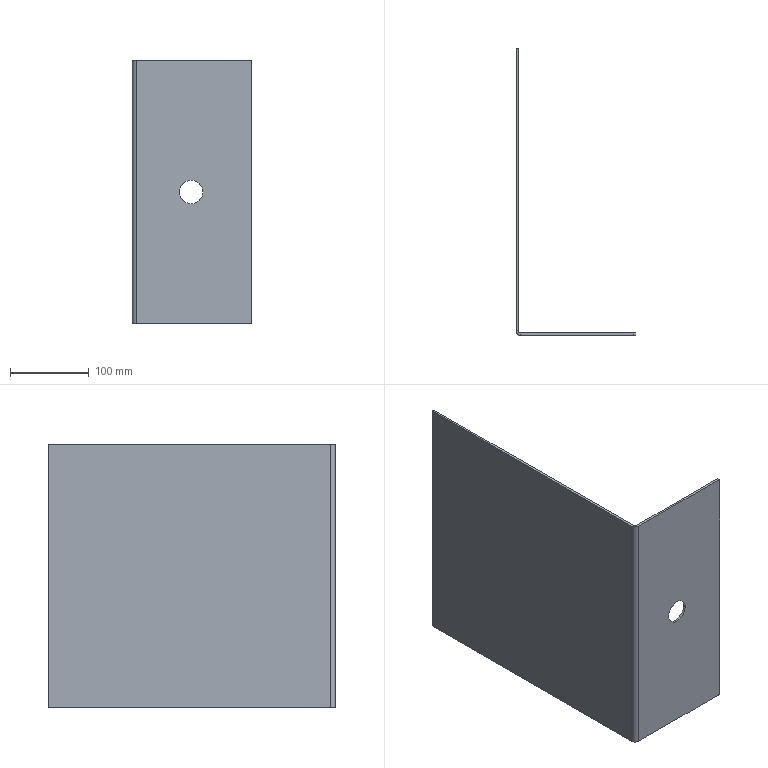Part | SolidWorks | features Cut 1, FlatPattern 1, ICE 1, SMBaseFlange 1, SheetMetal 1 | 1 solid | 18 faces | box 152 x 364 x 334 mm | volume 509961 mm3 | plane 12 | cylinder 6 | commonest cylinder face diameters 5.2 x2 30 x2 6 x1 12 x1
STEP:
#1=CARTESIAN_POINT('',(75.,3.,152.));
#2=VERTEX_POINT('',#1);
#3=CARTESIAN_POINT('',(75.,3.,182.));
#4=VERTEX_POINT('',#3);
#5=CARTESIAN_POINT('',(75.,3.,167.));
#6=DIRECTION('',(0.,1.,0.));
#7=DIRECTION('',(0.,0.,1.));
#8=AXIS2_PLACEMENT_3D('',#5,#6,#7);
#9=CIRCLE('',#8,15.);
#10=EDGE_CURVE('',#2,#4,#9,.T.);
#11=ORIENTED_EDGE('',*,*,#10,.T.);
#12=CARTESIAN_POINT('',(75.,0.,182.));
#13=VERTEX_POINT('',#12);
#14=CARTESIAN_POINT('',(75.,10.,182.));
#15=DIRECTION('',(0.,-1.,0.));
#16=VECTOR('',#15,1000.);
#17=LINE('',#14,#16);
#18=EDGE_CURVE('',#4,#13,#17,.T.);
#19=ORIENTED_EDGE('',*,*,#18,.T.);
#20=CARTESIAN_POINT('',(75.,0.,152.));
#21=VERTEX_POINT('',#20);
#22=CARTESIAN_POINT('',(75.,0.,167.));
#23=DIRECTION('',(0.,-1.,0.));
#24=DIRECTION('',(0.,0.,-1.));
#25=AXIS2_PLACEMENT_3D('',#22,#23,#24);
#26=CIRCLE('',#25,15.);
#27=EDGE_CURVE('',#13,#21,#26,.T.);
#28=ORIENTED_EDGE('',*,*,#27,.T.);
#29=CARTESIAN_POINT('',(75.,10.,152.));
#30=DIRECTION('',(0.,-1.,0.));
#31=VECTOR('',#30,1000.);
#32=LINE('',#29,#31);
#33=EDGE_CURVE('',#2,#21,#32,.T.);
#34=ORIENTED_EDGE('',*,*,#33,.F.);
#35=EDGE_LOOP('',(#11,#19,#28,#34));
#36=FACE_OUTER_BOUND('',#35,.T.);
#37=CARTESIAN_POINT('',(75.,10.,167.));
#38=DIRECTION('',(0.,-1.,0.));
#39=DIRECTION('',(0.,0.,-1.));
#40=AXIS2_PLACEMENT_3D('',#37,#38,#39);
#41=CYLINDRICAL_SURFACE('',#40,15.);
#42=ADVANCED_FACE('',(#36),#41,.F.);
#43=CARTESIAN_POINT('',(75.,0.,167.));
#44=DIRECTION('',(0.,-1.,0.));
#45=DIRECTION('',(0.,0.,-1.));
#46=AXIS2_PLACEMENT_3D('',#43,#44,#45);
#47=CIRCLE('',#46,15.);
#48=EDGE_CURVE('',#21,#13,#47,.T.);
#49=ORIENTED_EDGE('',*,*,#48,.F.);
#50=ORIENTED_EDGE('',*,*,#27,.F.);
#51=EDGE_LOOP('',(#49,#50));
#52=FACE_BOUND('',#51,.T.);
#53=CARTESIAN_POINT('',(149.4,0.,0.));
#54=VERTEX_POINT('',#53);
#55=CARTESIAN_POINT('',(152.,0.,2.6));
#56=VERTEX_POINT('',#55);
#57=CARTESIAN_POINT('',(149.4,0.,2.6));
#58=DIRECTION('',(0.,-1.,0.));
#59=DIRECTION('',(0.,0.,1.));
#60=AXIS2_PLACEMENT_3D('',#57,#58,#59);
#61=CIRCLE('',#60,2.6);
#62=EDGE_CURVE('',#54,#56,#61,.T.);
#63=ORIENTED_EDGE('',*,*,#62,.T.);
#64=CARTESIAN_POINT('',(152.,0.,331.4));
#65=VERTEX_POINT('',#64);
#66=CARTESIAN_POINT('',(152.,0.,334.));
#67=DIRECTION('',(0.,0.,-1.));
#68=VECTOR('',#67,1000.);
#69=LINE('',#66,#68);
#70=EDGE_CURVE('',#65,#56,#69,.T.);
#71=ORIENTED_EDGE('',*,*,#70,.F.);
#72=CARTESIAN_POINT('',(149.4,0.,334.));
#73=VERTEX_POINT('',#72);
#74=CARTESIAN_POINT('',(149.4,0.,331.4));
#75=DIRECTION('',(0.,-1.,0.));
#76=DIRECTION('',(0.,0.,1.));
#77=AXIS2_PLACEMENT_3D('',#74,#75,#76);
#78=CIRCLE('',#77,2.6);
#79=EDGE_CURVE('',#65,#73,#78,.T.);
#80=ORIENTED_EDGE('',*,*,#79,.T.);
#81=CARTESIAN_POINT('',(6.,0.,334.));
#82=VERTEX_POINT('',#81);
#83=CARTESIAN_POINT('',(0.,0.,334.));
#84=DIRECTION('',(1.,0.,0.));
#85=VECTOR('',#84,1000.);
#86=LINE('',#83,#85);
#87=EDGE_CURVE('',#82,#73,#86,.T.);
#88=ORIENTED_EDGE('',*,*,#87,.F.);
#89=CARTESIAN_POINT('',(6.,0.,0.));
#90=VERTEX_POINT('',#89);
#91=CARTESIAN_POINT('',(6.,0.,334.));
#92=DIRECTION('',(0.,0.,-1.));
#93=VECTOR('',#92,1000.);
#94=LINE('',#91,#93);
#95=EDGE_CURVE('',#82,#90,#94,.T.);
#96=ORIENTED_EDGE('',*,*,#95,.T.);
#97=CARTESIAN_POINT('',(0.,0.,0.));
#98=DIRECTION('',(1.,0.,0.));
#99=VECTOR('',#98,1000.);
#100=LINE('',#97,#99);
#101=EDGE_CURVE('',#90,#54,#100,.T.);
#102=ORIENTED_EDGE('',*,*,#101,.T.);
#103=EDGE_LOOP('',(#63,#71,#80,#88,#96,#102));
#104=FACE_OUTER_BOUND('',#103,.T.);
#105=CARTESIAN_POINT('',(0.,0.,334.));
#106=DIRECTION('',(0.,1.,0.));
#107=DIRECTION('',(0.,0.,1.));
#108=AXIS2_PLACEMENT_3D('',#105,#106,#107);
#109=PLANE('',#108);
#110=ADVANCED_FACE('',(#52,#104),#109,.F.);
#111=ORIENTED_EDGE('',*,*,#10,.F.);
#112=CARTESIAN_POINT('',(75.,3.,167.));
#113=DIRECTION('',(0.,1.,0.));
#114=DIRECTION('',(0.,0.,1.));
#115=AXIS2_PLACEMENT_3D('',#112,#113,#114);
#116=CIRCLE('',#115,15.);
#117=EDGE_CURVE('',#4,#2,#116,.T.);
#118=ORIENTED_EDGE('',*,*,#117,.F.);
#119=EDGE_LOOP('',(#111,#118));
#120=FACE_BOUND('',#119,.T.);
#121=CARTESIAN_POINT('',(152.,3.,331.4));
#122=VERTEX_POINT('',#121);
#123=CARTESIAN_POINT('',(152.,3.,2.6));
#124=VERTEX_POINT('',#123);
#125=CARTESIAN_POINT('',(152.,3.,334.));
#126=DIRECTION('',(0.,0.,-1.));
#127=VECTOR('',#126,1000.);
#128=LINE('',#125,#127);
#129=EDGE_CURVE('',#122,#124,#128,.T.);
#130=ORIENTED_EDGE('',*,*,#129,.T.);
#131=CARTESIAN_POINT('',(149.4,3.,0.));
#132=VERTEX_POINT('',#131);
#133=CARTESIAN_POINT('',(149.4,3.,2.6));
#134=DIRECTION('',(0.,-1.,0.));
#135=DIRECTION('',(0.,0.,1.));
#136=AXIS2_PLACEMENT_3D('',#133,#134,#135);
#137=CIRCLE('',#136,2.6);
#138=EDGE_CURVE('',#132,#124,#137,.T.);
#139=ORIENTED_EDGE('',*,*,#138,.F.);
#140=CARTESIAN_POINT('',(6.,3.,0.));
#141=VERTEX_POINT('',#140);
#142=CARTESIAN_POINT('',(0.,3.,0.));
#143=DIRECTION('',(1.,0.,0.));
#144=VECTOR('',#143,1000.);
#145=LINE('',#142,#144);
#146=EDGE_CURVE('',#141,#132,#145,.T.);
#147=ORIENTED_EDGE('',*,*,#146,.F.);
#148=CARTESIAN_POINT('',(6.,3.,334.));
#149=VERTEX_POINT('',#148);
#150=CARTESIAN_POINT('',(6.,3.,334.));
#151=DIRECTION('',(0.,0.,-1.));
#152=VECTOR('',#151,1000.);
#153=LINE('',#150,#152);
#154=EDGE_CURVE('',#149,#141,#153,.T.);
#155=ORIENTED_EDGE('',*,*,#154,.F.);
#156=CARTESIAN_POINT('',(149.4,3.,334.));
#157=VERTEX_POINT('',#156);
#158=CARTESIAN_POINT('',(0.,3.,334.));
#159=DIRECTION('',(1.,0.,0.));
#160=VECTOR('',#159,1000.);
#161=LINE('',#158,#160);
#162=EDGE_CURVE('',#149,#157,#161,.T.);
#163=ORIENTED_EDGE('',*,*,#162,.T.);
#164=CARTESIAN_POINT('',(149.4,3.,331.4));
#165=DIRECTION('',(0.,-1.,0.));
#166=DIRECTION('',(0.,0.,1.));
#167=AXIS2_PLACEMENT_3D('',#164,#165,#166);
#168=CIRCLE('',#167,2.6);
#169=EDGE_CURVE('',#122,#157,#168,.T.);
#170=ORIENTED_EDGE('',*,*,#169,.F.);
#171=EDGE_LOOP('',(#130,#139,#147,#155,#163,#170));
#172=FACE_OUTER_BOUND('',#171,.T.);
#173=CARTESIAN_POINT('',(0.,3.,334.));
#174=DIRECTION('',(0.,1.,0.));
#175=DIRECTION('',(0.,0.,1.));
#176=AXIS2_PLACEMENT_3D('',#173,#174,#175);
#177=PLANE('',#176);
#178=ADVANCED_FACE('',(#120,#172),#177,.T.);
#179=ORIENTED_EDGE('',*,*,#70,.T.);
#180=CARTESIAN_POINT('',(152.,3.,2.6));
#181=DIRECTION('',(0.,-1.,0.));
#182=VECTOR('',#181,1000.);
#183=LINE('',#180,#182);
#184=EDGE_CURVE('',#124,#56,#183,.T.);
#185=ORIENTED_EDGE('',*,*,#184,.F.);
#186=ORIENTED_EDGE('',*,*,#129,.F.);
#187=CARTESIAN_POINT('',(152.,3.,331.4));
#188=DIRECTION('',(0.,-1.,0.));
#189=VECTOR('',#188,1000.);
#190=LINE('',#187,#189);
#191=EDGE_CURVE('',#122,#65,#190,.T.);
#192=ORIENTED_EDGE('',*,*,#191,.T.);
#193=EDGE_LOOP('',(#179,#185,#186,#192));
#194=FACE_OUTER_BOUND('',#193,.T.);
#195=CARTESIAN_POINT('',(152.,3.,334.));
#196=DIRECTION('',(1.,0.,0.));
#197=DIRECTION('',(0.,0.,-1.));
#198=AXIS2_PLACEMENT_3D('',#195,#196,#197);
#199=PLANE('',#198);
#200=ADVANCED_FACE('',(#194),#199,.T.);
#201=ORIENTED_EDGE('',*,*,#87,.T.);
#202=CARTESIAN_POINT('',(149.4,3.,334.));
#203=DIRECTION('',(0.,-1.,0.));
#204=VECTOR('',#203,1000.);
#205=LINE('',#202,#204);
#206=EDGE_CURVE('',#157,#73,#205,.T.);
#207=ORIENTED_EDGE('',*,*,#206,.F.);
#208=ORIENTED_EDGE('',*,*,#162,.F.);
#209=CARTESIAN_POINT('',(6.,3.,334.));
#210=DIRECTION('',(0.,-1.,0.));
#211=VECTOR('',#210,1000.);
#212=LINE('',#209,#211);
#213=EDGE_CURVE('',#149,#82,#212,.T.);
#214=ORIENTED_EDGE('',*,*,#213,.T.);
#215=EDGE_LOOP('',(#201,#207,#208,#214));
#216=FACE_OUTER_BOUND('',#215,.T.);
#217=CARTESIAN_POINT('',(6.,6.,334.));
#218=DIRECTION('',(0.,0.,1.));
#219=DIRECTION('',(1.,0.,0.));
#220=AXIS2_PLACEMENT_3D('',#217,#218,#219);
#221=PLANE('',#220);
#222=ADVANCED_FACE('',(#216),#221,.T.);
#223=CARTESIAN_POINT('',(0.,6.,334.));
#224=VERTEX_POINT('',#223);
#225=CARTESIAN_POINT('',(3.,6.,334.));
#226=VERTEX_POINT('',#225);
#227=CARTESIAN_POINT('',(0.,6.,334.));
#228=DIRECTION('',(1.,0.,0.));
#229=VECTOR('',#228,1000.);
#230=LINE('',#227,#229);
#231=EDGE_CURVE('',#224,#226,#230,.T.);
#232=ORIENTED_EDGE('',*,*,#231,.F.);
#233=CARTESIAN_POINT('',(6.,6.,334.));
#234=DIRECTION('',(0.,0.,1.));
#235=DIRECTION('',(-1.,0.,0.));
#236=AXIS2_PLACEMENT_3D('',#233,#234,#235);
#237=CIRCLE('',#236,6.);
#238=EDGE_CURVE('',#224,#82,#237,.T.);
#239=ORIENTED_EDGE('',*,*,#238,.T.);
#240=ORIENTED_EDGE('',*,*,#213,.F.);
#241=CARTESIAN_POINT('',(6.,6.,334.));
#242=DIRECTION('',(0.,0.,1.));
#243=DIRECTION('',(1.,0.,0.));
#244=AXIS2_PLACEMENT_3D('',#241,#242,#243);
#245=CIRCLE('',#244,3.);
#246=EDGE_CURVE('',#226,#149,#245,.T.);
#247=ORIENTED_EDGE('',*,*,#246,.F.);
#248=EDGE_LOOP('',(#232,#239,#240,#247));
#249=FACE_OUTER_BOUND('',#248,.T.);
#250=CARTESIAN_POINT('',(0.,6.,334.));
#251=DIRECTION('',(0.,0.,1.));
#252=DIRECTION('',(1.,0.,0.));
#253=AXIS2_PLACEMENT_3D('',#250,#251,#252);
#254=PLANE('',#253);
#255=ADVANCED_FACE('',(#249),#254,.T.);
#256=CARTESIAN_POINT('',(0.,364.,334.));
#257=VERTEX_POINT('',#256);
#258=CARTESIAN_POINT('',(0.,0.,334.));
#259=DIRECTION('',(0.,-1.,0.));
#260=VECTOR('',#259,1000.);
#261=LINE('',#258,#260);
#262=EDGE_CURVE('',#257,#224,#261,.T.);
#263=ORIENTED_EDGE('',*,*,#262,.T.);
#264=ORIENTED_EDGE('',*,*,#231,.T.);
#265=CARTESIAN_POINT('',(3.,364.,334.));
#266=VERTEX_POINT('',#265);
#267=CARTESIAN_POINT('',(3.,0.,334.));
#268=DIRECTION('',(0.,-1.,0.));
#269=VECTOR('',#268,1000.);
#270=LINE('',#267,#269);
#271=EDGE_CURVE('',#266,#226,#270,.T.);
#272=ORIENTED_EDGE('',*,*,#271,.F.);
#273=CARTESIAN_POINT('',(0.,364.,334.));
#274=DIRECTION('',(1.,0.,0.));
#275=VECTOR('',#274,1000.);
#276=LINE('',#273,#275);
#277=EDGE_CURVE('',#257,#266,#276,.T.);
#278=ORIENTED_EDGE('',*,*,#277,.F.);
#279=EDGE_LOOP('',(#263,#264,#272,#278));
#280=FACE_OUTER_BOUND('',#279,.T.);
#281=CARTESIAN_POINT('',(6.,3.,334.));
#282=DIRECTION('',(0.,0.,1.));
#283=DIRECTION('',(1.,0.,0.));
#284=AXIS2_PLACEMENT_3D('',#281,#282,#283);
#285=PLANE('',#284);
#286=ADVANCED_FACE('',(#280),#285,.T.);
#287=CARTESIAN_POINT('',(6.,0.,0.));
#288=DIRECTION('',(0.,1.,0.));
#289=VECTOR('',#288,1000.);
#290=LINE('',#287,#289);
#291=EDGE_CURVE('',#90,#141,#290,.T.);
#292=ORIENTED_EDGE('',*,*,#291,.F.);
#293=CARTESIAN_POINT('',(0.,6.,0.));
#294=VERTEX_POINT('',#293);
#295=CARTESIAN_POINT('',(6.,6.,0.));
#296=DIRECTION('',(0.,0.,1.));
#297=DIRECTION('',(-1.,0.,0.));
#298=AXIS2_PLACEMENT_3D('',#295,#296,#297);
#299=CIRCLE('',#298,6.);
#300=EDGE_CURVE('',#294,#90,#299,.T.);
#301=ORIENTED_EDGE('',*,*,#300,.F.);
#302=CARTESIAN_POINT('',(3.,6.,0.));
#303=VERTEX_POINT('',#302);
#304=CARTESIAN_POINT('',(3.,6.,0.));
#305=DIRECTION('',(-1.,0.,0.));
#306=VECTOR('',#305,1000.);
#307=LINE('',#304,#306);
#308=EDGE_CURVE('',#303,#294,#307,.T.);
#309=ORIENTED_EDGE('',*,*,#308,.F.);
#310=CARTESIAN_POINT('',(6.,6.,0.));
#311=DIRECTION('',(0.,0.,1.));
#312=DIRECTION('',(1.,0.,0.));
#313=AXIS2_PLACEMENT_3D('',#310,#311,#312);
#314=CIRCLE('',#313,3.);
#315=EDGE_CURVE('',#303,#141,#314,.T.);
#316=ORIENTED_EDGE('',*,*,#315,.T.);
#317=EDGE_LOOP('',(#292,#301,#309,#316));
#318=FACE_OUTER_BOUND('',#317,.T.);
#319=CARTESIAN_POINT('',(6.,0.,0.));
#320=DIRECTION('',(0.,0.,-1.));
#321=DIRECTION('',(-1.,0.,0.));
#322=AXIS2_PLACEMENT_3D('',#319,#320,#321);
#323=PLANE('',#322);
#324=ADVANCED_FACE('',(#318),#323,.T.);
#325=CARTESIAN_POINT('',(149.4,3.,0.));
#326=DIRECTION('',(0.,-1.,0.));
#327=VECTOR('',#326,1000.);
#328=LINE('',#325,#327);
#329=EDGE_CURVE('',#132,#54,#328,.T.);
#330=ORIENTED_EDGE('',*,*,#329,.T.);
#331=ORIENTED_EDGE('',*,*,#101,.F.);
#332=ORIENTED_EDGE('',*,*,#291,.T.);
#333=ORIENTED_EDGE('',*,*,#146,.T.);
#334=EDGE_LOOP('',(#330,#331,#332,#333));
#335=FACE_OUTER_BOUND('',#334,.T.);
#336=CARTESIAN_POINT('',(3.,6.,0.));
#337=DIRECTION('',(0.,0.,-1.));
#338=DIRECTION('',(-1.,0.,0.));
#339=AXIS2_PLACEMENT_3D('',#336,#337,#338);
#340=PLANE('',#339);
#341=ADVANCED_FACE('',(#335),#340,.T.);
#342=ORIENTED_EDGE('',*,*,#315,.F.);
#343=CARTESIAN_POINT('',(3.,6.,334.));
#344=DIRECTION('',(0.,0.,-1.));
#345=VECTOR('',#344,1000.);
#346=LINE('',#343,#345);
#347=EDGE_CURVE('',#226,#303,#346,.T.);
#348=ORIENTED_EDGE('',*,*,#347,.F.);
#349=ORIENTED_EDGE('',*,*,#246,.T.);
#350=ORIENTED_EDGE('',*,*,#154,.T.);
#351=EDGE_LOOP('',(#342,#348,#349,#350));
#352=FACE_OUTER_BOUND('',#351,.T.);
#353=CARTESIAN_POINT('',(6.,6.,334.));
#354=DIRECTION('',(0.,0.,-1.));
#355=DIRECTION('',(-1.,0.,0.));
#356=AXIS2_PLACEMENT_3D('',#353,#354,#355);
#357=CYLINDRICAL_SURFACE('',#356,3.);
#358=ADVANCED_FACE('',(#352),#357,.F.);
#359=CARTESIAN_POINT('',(3.,364.,0.));
#360=VERTEX_POINT('',#359);
#361=CARTESIAN_POINT('',(3.,0.,0.));
#362=DIRECTION('',(0.,-1.,0.));
#363=VECTOR('',#362,1000.);
#364=LINE('',#361,#363);
#365=EDGE_CURVE('',#360,#303,#364,.T.);
#366=ORIENTED_EDGE('',*,*,#365,.F.);
#367=CARTESIAN_POINT('',(3.,364.,334.));
#368=DIRECTION('',(0.,0.,-1.));
#369=VECTOR('',#368,1000.);
#370=LINE('',#367,#369);
#371=EDGE_CURVE('',#266,#360,#370,.T.);
#372=ORIENTED_EDGE('',*,*,#371,.F.);
#373=ORIENTED_EDGE('',*,*,#271,.T.);
#374=ORIENTED_EDGE('',*,*,#347,.T.);
#375=EDGE_LOOP('',(#366,#372,#373,#374));
#376=FACE_OUTER_BOUND('',#375,.T.);
#377=CARTESIAN_POINT('',(3.,0.,334.));
#378=DIRECTION('',(1.,0.,0.));
#379=DIRECTION('',(0.,0.,-1.));
#380=AXIS2_PLACEMENT_3D('',#377,#378,#379);
#381=PLANE('',#380);
#382=ADVANCED_FACE('',(#376),#381,.T.);
#383=CARTESIAN_POINT('',(0.,364.,0.));
#384=VERTEX_POINT('',#383);
#385=CARTESIAN_POINT('',(0.,364.,0.));
#386=DIRECTION('',(1.,0.,0.));
#387=VECTOR('',#386,1000.);
#388=LINE('',#385,#387);
#389=EDGE_CURVE('',#384,#360,#388,.T.);
#390=ORIENTED_EDGE('',*,*,#389,.F.);
#391=CARTESIAN_POINT('',(0.,364.,334.));
#392=DIRECTION('',(0.,0.,-1.));
#393=VECTOR('',#392,1000.);
#394=LINE('',#391,#393);
#395=EDGE_CURVE('',#257,#384,#394,.T.);
#396=ORIENTED_EDGE('',*,*,#395,.F.);
#397=ORIENTED_EDGE('',*,*,#277,.T.);
#398=ORIENTED_EDGE('',*,*,#371,.T.);
#399=EDGE_LOOP('',(#390,#396,#397,#398));
#400=FACE_OUTER_BOUND('',#399,.T.);
#401=CARTESIAN_POINT('',(0.,364.,334.));
#402=DIRECTION('',(0.,1.,0.));
#403=DIRECTION('',(0.,0.,1.));
#404=AXIS2_PLACEMENT_3D('',#401,#402,#403);
#405=PLANE('',#404);
#406=ADVANCED_FACE('',(#400),#405,.T.);
#407=CARTESIAN_POINT('',(0.,0.,0.));
#408=DIRECTION('',(0.,-1.,0.));
#409=VECTOR('',#408,1000.);
#410=LINE('',#407,#409);
#411=EDGE_CURVE('',#384,#294,#410,.T.);
#412=ORIENTED_EDGE('',*,*,#411,.T.);
#413=CARTESIAN_POINT('',(0.,6.,334.));
#414=DIRECTION('',(0.,0.,-1.));
#415=VECTOR('',#414,1000.);
#416=LINE('',#413,#415);
#417=EDGE_CURVE('',#224,#294,#416,.T.);
#418=ORIENTED_EDGE('',*,*,#417,.F.);
#419=ORIENTED_EDGE('',*,*,#262,.F.);
#420=ORIENTED_EDGE('',*,*,#395,.T.);
#421=EDGE_LOOP('',(#412,#418,#419,#420));
#422=FACE_OUTER_BOUND('',#421,.T.);
#423=CARTESIAN_POINT('',(0.,0.,334.));
#424=DIRECTION('',(1.,0.,0.));
#425=DIRECTION('',(0.,0.,-1.));
#426=AXIS2_PLACEMENT_3D('',#423,#424,#425);
#427=PLANE('',#426);
#428=ADVANCED_FACE('',(#422),#427,.F.);
#429=ORIENTED_EDGE('',*,*,#300,.T.);
#430=ORIENTED_EDGE('',*,*,#95,.F.);
#431=ORIENTED_EDGE('',*,*,#238,.F.);
#432=ORIENTED_EDGE('',*,*,#417,.T.);
#433=EDGE_LOOP('',(#429,#430,#431,#432));
#434=FACE_OUTER_BOUND('',#433,.T.);
#435=CARTESIAN_POINT('',(6.,6.,334.));
#436=DIRECTION('',(0.,0.,-1.));
#437=DIRECTION('',(-1.,0.,0.));
#438=AXIS2_PLACEMENT_3D('',#435,#436,#437);
#439=CYLINDRICAL_SURFACE('',#438,6.);
#440=ADVANCED_FACE('',(#434),#439,.T.);
#441=ORIENTED_EDGE('',*,*,#365,.T.);
#442=ORIENTED_EDGE('',*,*,#308,.T.);
#443=ORIENTED_EDGE('',*,*,#411,.F.);
#444=ORIENTED_EDGE('',*,*,#389,.T.);
#445=EDGE_LOOP('',(#441,#442,#443,#444));
#446=FACE_OUTER_BOUND('',#445,.T.);
#447=CARTESIAN_POINT('',(6.,6.,0.));
#448=DIRECTION('',(0.,0.,1.));
#449=DIRECTION('',(1.,0.,0.));
#450=AXIS2_PLACEMENT_3D('',#447,#448,#449);
#451=PLANE('',#450);
#452=ADVANCED_FACE('',(#446),#451,.F.);
#453=ORIENTED_EDGE('',*,*,#169,.T.);
#454=ORIENTED_EDGE('',*,*,#206,.T.);
#455=ORIENTED_EDGE('',*,*,#79,.F.);
#456=ORIENTED_EDGE('',*,*,#191,.F.);
#457=EDGE_LOOP('',(#453,#454,#455,#456));
#458=FACE_OUTER_BOUND('',#457,.T.);
#459=CARTESIAN_POINT('',(149.4,3.,331.4));
#460=DIRECTION('',(0.,1.,0.));
#461=DIRECTION('',(0.,0.,1.));
#462=AXIS2_PLACEMENT_3D('',#459,#460,#461);
#463=CYLINDRICAL_SURFACE('',#462,2.6);
#464=ADVANCED_FACE('',(#458),#463,.T.);
#465=ORIENTED_EDGE('',*,*,#138,.T.);
#466=ORIENTED_EDGE('',*,*,#184,.T.);
#467=ORIENTED_EDGE('',*,*,#62,.F.);
#468=ORIENTED_EDGE('',*,*,#329,.F.);
#469=EDGE_LOOP('',(#465,#466,#467,#468));
#470=FACE_OUTER_BOUND('',#469,.T.);
#471=CARTESIAN_POINT('',(149.4,3.,2.6));
#472=DIRECTION('',(0.,1.,0.));
#473=DIRECTION('',(0.,0.,1.));
#474=AXIS2_PLACEMENT_3D('',#471,#472,#473);
#475=CYLINDRICAL_SURFACE('',#474,2.6);
#476=ADVANCED_FACE('',(#470),#475,.T.);
#477=ORIENTED_EDGE('',*,*,#18,.F.);
#478=ORIENTED_EDGE('',*,*,#117,.T.);
#479=ORIENTED_EDGE('',*,*,#33,.T.);
#480=ORIENTED_EDGE('',*,*,#48,.T.);
#481=EDGE_LOOP('',(#477,#478,#479,#480));
#482=FACE_OUTER_BOUND('',#481,.T.);
#483=CARTESIAN_POINT('',(75.,10.,167.));
#484=DIRECTION('',(0.,-1.,0.));
#485=DIRECTION('',(0.,0.,-1.));
#486=AXIS2_PLACEMENT_3D('',#483,#484,#485);
#487=CYLINDRICAL_SURFACE('',#486,15.);
#488=ADVANCED_FACE('',(#482),#487,.F.);
#489=CLOSED_SHELL('',(#42,#110,#178,#200,#222,#255,#286,#324,#341,#358,#382,#406,#428,#440,#452,#464,#476,#488));
#490=MANIFOLD_SOLID_BREP('',#489);
#491=CARTESIAN_POINT('',(0.,0.,0.));
#492=DIRECTION('',(0.,0.,1.));
#493=DIRECTION('',(1.,0.,0.));
#494=AXIS2_PLACEMENT_3D('',#491,#492,#493);
#495=(LENGTH_UNIT()NAMED_UNIT(*)SI_UNIT(.MILLI.,.METRE.));
#496=UNCERTAINTY_MEASURE_WITH_UNIT(LENGTH_MEASURE(0.00001),#495,'','');
#497=(NAMED_UNIT(*)PLANE_ANGLE_UNIT()SI_UNIT($,.RADIAN.));
#498=(NAMED_UNIT(*)SI_UNIT($,.STERADIAN.)SOLID_ANGLE_UNIT());
#499=(GEOMETRIC_REPRESENTATION_CONTEXT(3)GLOBAL_UNCERTAINTY_ASSIGNED_CONTEXT((#496))GLOBAL_UNIT_ASSIGNED_CONTEXT((#495,#497,#498))REPRESENTATION_CONTEXT('',''));
#500=ADVANCED_BREP_SHAPE_REPRESENTATION('',(#490,#494),#499);